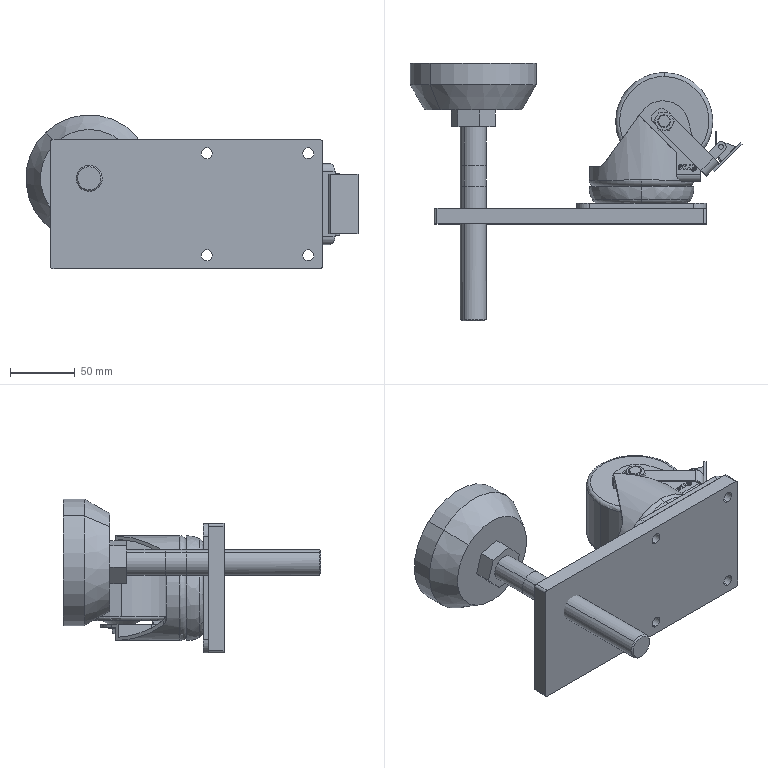Part | SolidWorks | 5 solids | 288 faces | box 256.604 x 199 x 119 mm | volume 916637 mm3 | plane 150 | cylinder 83 | cone 35 | torus 10 | spline 10 | commonest cylinder face diameters 10 x22 11 x12 4 x10 20 x10 8.5 x8 8 x5